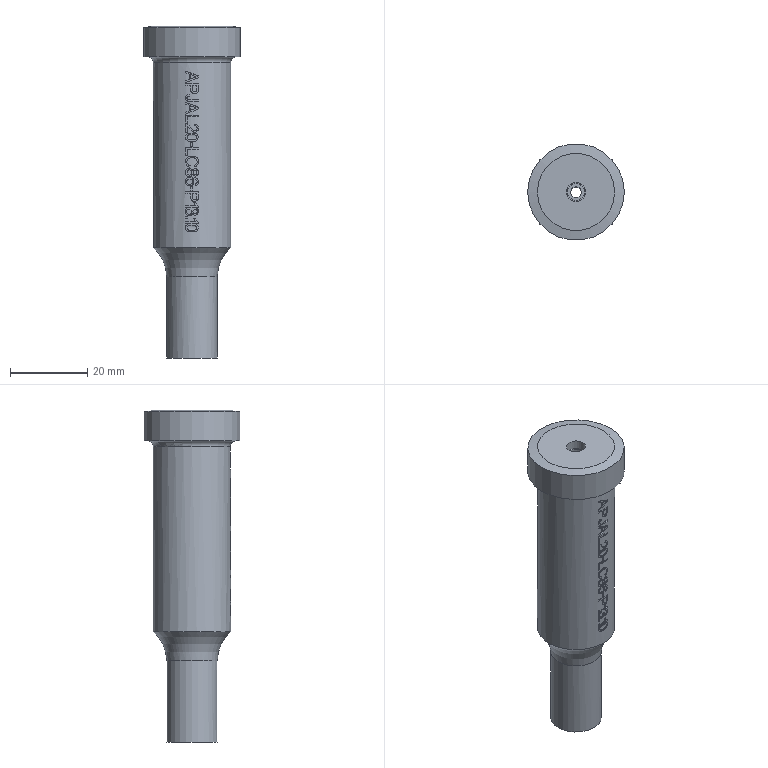Part | NX | features MI_APJAL_0242 2 | 1 solid | 226 faces | box 25 x 25 x 86 mm | volume 22683 mm3 | plane 128 | cylinder 95 | torus 2 | cone 1 | commonest cylinder face diameters 19.8 x19 20 x10 1.066 x2 1.174 x2 1.332 x2 1.395 x2